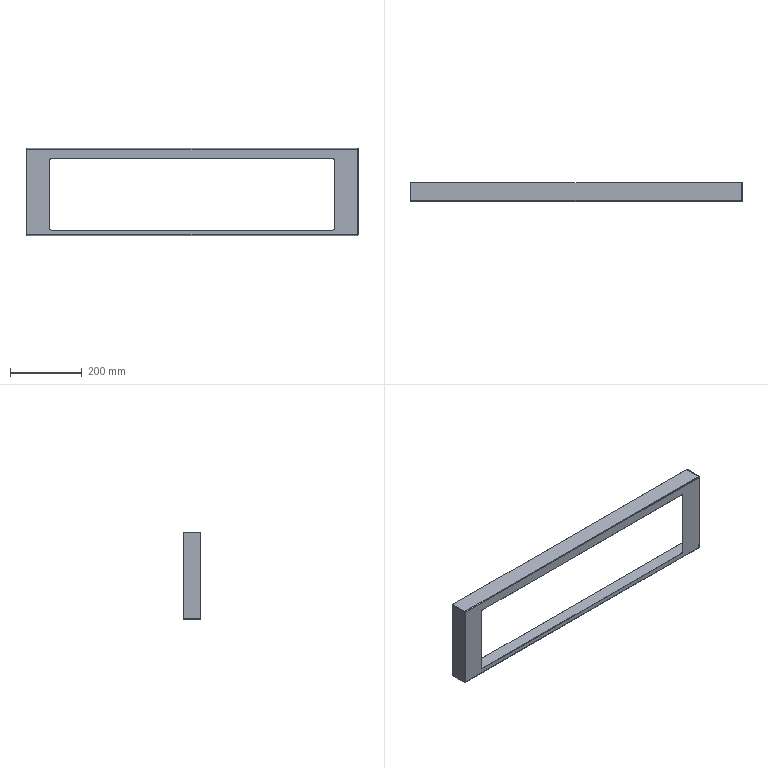Part | SolidWorks | features BaseBody 1 | 1 solid | 48 faces | box 927 x 50 x 243 mm | volume 213988 mm3 | plane 36 | cylinder 12 | commonest cylinder face diameters 2 x4 4.4 x4 10 x4
STEP:
#1=CARTESIAN_POINT('',(392.5,-23.8,13.8));
#2=VERTEX_POINT('',#1);
#3=CARTESIAN_POINT('',(397.5,-23.8,18.8));
#4=VERTEX_POINT('',#3);
#5=CARTESIAN_POINT('',(392.5,-23.8,18.8));
#6=DIRECTION('',(0.,-1.,0.));
#7=DIRECTION('',(0.,0.,1.));
#8=AXIS2_PLACEMENT_3D('',#5,#6,#7);
#9=CIRCLE('',#8,5.);
#10=EDGE_CURVE('',#2,#4,#9,.T.);
#11=ORIENTED_EDGE('',*,*,#10,.F.);
#12=CARTESIAN_POINT('',(392.5,-25.,13.8));
#13=VERTEX_POINT('',#12);
#14=CARTESIAN_POINT('',(392.5,-23.8,13.8));
#15=DIRECTION('',(0.,1.,0.));
#16=VECTOR('',#15,1000.);
#17=LINE('',#14,#16);
#18=EDGE_CURVE('',#13,#2,#17,.T.);
#19=ORIENTED_EDGE('',*,*,#18,.F.);
#20=CARTESIAN_POINT('',(397.5,-25.,18.8));
#21=VERTEX_POINT('',#20);
#22=CARTESIAN_POINT('',(392.5,-25.,18.8));
#23=DIRECTION('',(0.,1.,0.));
#24=DIRECTION('',(0.,0.,1.));
#25=AXIS2_PLACEMENT_3D('',#22,#23,#24);
#26=CIRCLE('',#25,5.);
#27=EDGE_CURVE('',#21,#13,#26,.T.);
#28=ORIENTED_EDGE('',*,*,#27,.F.);
#29=CARTESIAN_POINT('',(397.5,-25.,18.8));
#30=DIRECTION('',(0.,-1.,0.));
#31=VECTOR('',#30,1000.);
#32=LINE('',#29,#31);
#33=EDGE_CURVE('',#4,#21,#32,.T.);
#34=ORIENTED_EDGE('',*,*,#33,.F.);
#35=EDGE_LOOP('',(#11,#19,#28,#34));
#36=FACE_OUTER_BOUND('',#35,.T.);
#37=CARTESIAN_POINT('',(392.5,-15.,18.8));
#38=DIRECTION('',(0.,1.,0.));
#39=DIRECTION('',(0.,0.,1.));
#40=AXIS2_PLACEMENT_3D('',#37,#38,#39);
#41=CYLINDRICAL_SURFACE('',#40,5.);
#42=ADVANCED_FACE('',(#36),#41,.F.);
#43=CARTESIAN_POINT('',(-397.5,-23.8,18.8));
#44=VERTEX_POINT('',#43);
#45=CARTESIAN_POINT('',(-392.5,-23.8,13.8));
#46=VERTEX_POINT('',#45);
#47=CARTESIAN_POINT('',(-392.5,-23.8,18.8));
#48=DIRECTION('',(0.,-1.,0.));
#49=DIRECTION('',(0.,0.,1.));
#50=AXIS2_PLACEMENT_3D('',#47,#48,#49);
#51=CIRCLE('',#50,5.);
#52=EDGE_CURVE('',#44,#46,#51,.T.);
#53=ORIENTED_EDGE('',*,*,#52,.F.);
#54=CARTESIAN_POINT('',(-397.5,-25.,18.8));
#55=VERTEX_POINT('',#54);
#56=CARTESIAN_POINT('',(-397.5,-23.8,18.8));
#57=DIRECTION('',(0.,1.,0.));
#58=VECTOR('',#57,1000.);
#59=LINE('',#56,#58);
#60=EDGE_CURVE('',#55,#44,#59,.T.);
#61=ORIENTED_EDGE('',*,*,#60,.F.);
#62=CARTESIAN_POINT('',(-392.5,-25.,13.8));
#63=VERTEX_POINT('',#62);
#64=CARTESIAN_POINT('',(-392.5,-25.,18.8));
#65=DIRECTION('',(0.,1.,0.));
#66=DIRECTION('',(0.,0.,1.));
#67=AXIS2_PLACEMENT_3D('',#64,#65,#66);
#68=CIRCLE('',#67,5.);
#69=EDGE_CURVE('',#63,#55,#68,.T.);
#70=ORIENTED_EDGE('',*,*,#69,.F.);
#71=CARTESIAN_POINT('',(-392.5,-25.,13.8));
#72=DIRECTION('',(0.,-1.,0.));
#73=VECTOR('',#72,1000.);
#74=LINE('',#71,#73);
#75=EDGE_CURVE('',#46,#63,#74,.T.);
#76=ORIENTED_EDGE('',*,*,#75,.F.);
#77=EDGE_LOOP('',(#53,#61,#70,#76));
#78=FACE_OUTER_BOUND('',#77,.T.);
#79=CARTESIAN_POINT('',(-392.5,-15.,18.8));
#80=DIRECTION('',(0.,1.,0.));
#81=DIRECTION('',(0.,0.,1.));
#82=AXIS2_PLACEMENT_3D('',#79,#80,#81);
#83=CYLINDRICAL_SURFACE('',#82,5.);
#84=ADVANCED_FACE('',(#78),#83,.F.);
#85=CARTESIAN_POINT('',(-392.5,-23.8,213.8));
#86=VERTEX_POINT('',#85);
#87=CARTESIAN_POINT('',(-397.5,-23.8,208.8));
#88=VERTEX_POINT('',#87);
#89=CARTESIAN_POINT('',(-392.5,-23.8,208.8));
#90=DIRECTION('',(0.,-1.,0.));
#91=DIRECTION('',(0.,0.,1.));
#92=AXIS2_PLACEMENT_3D('',#89,#90,#91);
#93=CIRCLE('',#92,5.);
#94=EDGE_CURVE('',#86,#88,#93,.T.);
#95=ORIENTED_EDGE('',*,*,#94,.F.);
#96=CARTESIAN_POINT('',(-392.5,-25.,213.8));
#97=VERTEX_POINT('',#96);
#98=CARTESIAN_POINT('',(-392.5,-23.8,213.8));
#99=DIRECTION('',(0.,1.,0.));
#100=VECTOR('',#99,1000.);
#101=LINE('',#98,#100);
#102=EDGE_CURVE('',#97,#86,#101,.T.);
#103=ORIENTED_EDGE('',*,*,#102,.F.);
#104=CARTESIAN_POINT('',(-397.5,-25.,208.8));
#105=VERTEX_POINT('',#104);
#106=CARTESIAN_POINT('',(-392.5,-25.,208.8));
#107=DIRECTION('',(0.,1.,0.));
#108=DIRECTION('',(0.,0.,1.));
#109=AXIS2_PLACEMENT_3D('',#106,#107,#108);
#110=CIRCLE('',#109,5.);
#111=EDGE_CURVE('',#105,#97,#110,.T.);
#112=ORIENTED_EDGE('',*,*,#111,.F.);
#113=CARTESIAN_POINT('',(-397.5,-25.,208.8));
#114=DIRECTION('',(0.,-1.,0.));
#115=VECTOR('',#114,1000.);
#116=LINE('',#113,#115);
#117=EDGE_CURVE('',#88,#105,#116,.T.);
#118=ORIENTED_EDGE('',*,*,#117,.F.);
#119=EDGE_LOOP('',(#95,#103,#112,#118));
#120=FACE_OUTER_BOUND('',#119,.T.);
#121=CARTESIAN_POINT('',(-392.5,-15.,208.8));
#122=DIRECTION('',(0.,1.,0.));
#123=DIRECTION('',(0.,0.,1.));
#124=AXIS2_PLACEMENT_3D('',#121,#122,#123);
#125=CYLINDRICAL_SURFACE('',#124,5.);
#126=ADVANCED_FACE('',(#120),#125,.F.);
#127=CARTESIAN_POINT('',(397.5,-23.8,208.8));
#128=VERTEX_POINT('',#127);
#129=CARTESIAN_POINT('',(392.5,-23.8,213.8));
#130=VERTEX_POINT('',#129);
#131=CARTESIAN_POINT('',(392.5,-23.8,208.8));
#132=DIRECTION('',(0.,-1.,0.));
#133=DIRECTION('',(0.,0.,1.));
#134=AXIS2_PLACEMENT_3D('',#131,#132,#133);
#135=CIRCLE('',#134,5.);
#136=EDGE_CURVE('',#128,#130,#135,.T.);
#137=ORIENTED_EDGE('',*,*,#136,.F.);
#138=CARTESIAN_POINT('',(397.5,-25.,208.8));
#139=VERTEX_POINT('',#138);
#140=CARTESIAN_POINT('',(397.5,-23.8,208.8));
#141=DIRECTION('',(0.,1.,0.));
#142=VECTOR('',#141,1000.);
#143=LINE('',#140,#142);
#144=EDGE_CURVE('',#139,#128,#143,.T.);
#145=ORIENTED_EDGE('',*,*,#144,.F.);
#146=CARTESIAN_POINT('',(392.5,-25.,213.8));
#147=VERTEX_POINT('',#146);
#148=CARTESIAN_POINT('',(392.5,-25.,208.8));
#149=DIRECTION('',(0.,1.,0.));
#150=DIRECTION('',(0.,0.,1.));
#151=AXIS2_PLACEMENT_3D('',#148,#149,#150);
#152=CIRCLE('',#151,5.);
#153=EDGE_CURVE('',#147,#139,#152,.T.);
#154=ORIENTED_EDGE('',*,*,#153,.F.);
#155=CARTESIAN_POINT('',(392.5,-25.,213.8));
#156=DIRECTION('',(0.,-1.,0.));
#157=VECTOR('',#156,1000.);
#158=LINE('',#155,#157);
#159=EDGE_CURVE('',#130,#147,#158,.T.);
#160=ORIENTED_EDGE('',*,*,#159,.F.);
#161=EDGE_LOOP('',(#137,#145,#154,#160));
#162=FACE_OUTER_BOUND('',#161,.T.);
#163=CARTESIAN_POINT('',(392.5,-15.,208.8));
#164=DIRECTION('',(0.,1.,0.));
#165=DIRECTION('',(0.,0.,1.));
#166=AXIS2_PLACEMENT_3D('',#163,#164,#165);
#167=CYLINDRICAL_SURFACE('',#166,5.);
#168=ADVANCED_FACE('',(#162),#167,.F.);
#169=CARTESIAN_POINT('',(0.,-23.8,13.8));
#170=DIRECTION('',(-1.,0.,0.));
#171=VECTOR('',#170,1000.);
#172=LINE('',#169,#171);
#173=EDGE_CURVE('',#2,#46,#172,.T.);
#174=ORIENTED_EDGE('',*,*,#173,.T.);
#175=ORIENTED_EDGE('',*,*,#75,.T.);
#176=CARTESIAN_POINT('',(397.5,-25.,13.8));
#177=DIRECTION('',(1.,0.,0.));
#178=VECTOR('',#177,1000.);
#179=LINE('',#176,#178);
#180=EDGE_CURVE('',#63,#13,#179,.T.);
#181=ORIENTED_EDGE('',*,*,#180,.T.);
#182=ORIENTED_EDGE('',*,*,#18,.T.);
#183=EDGE_LOOP('',(#174,#175,#181,#182));
#184=FACE_OUTER_BOUND('',#183,.T.);
#185=CARTESIAN_POINT('',(397.5,-15.,13.8));
#186=DIRECTION('',(0.,0.,-1.));
#187=DIRECTION('',(-1.,0.,0.));
#188=AXIS2_PLACEMENT_3D('',#185,#186,#187);
#189=PLANE('',#188);
#190=ADVANCED_FACE('',(#184),#189,.F.);
#191=CARTESIAN_POINT('',(397.5,-25.,213.8));
#192=DIRECTION('',(0.,0.,1.));
#193=VECTOR('',#192,1000.);
#194=LINE('',#191,#193);
#195=EDGE_CURVE('',#21,#139,#194,.T.);
#196=ORIENTED_EDGE('',*,*,#195,.T.);
#197=ORIENTED_EDGE('',*,*,#144,.T.);
#198=CARTESIAN_POINT('',(397.5,-23.8,0.));
#199=DIRECTION('',(0.,0.,-1.));
#200=VECTOR('',#199,1000.);
#201=LINE('',#198,#200);
#202=EDGE_CURVE('',#128,#4,#201,.T.);
#203=ORIENTED_EDGE('',*,*,#202,.T.);
#204=ORIENTED_EDGE('',*,*,#33,.T.);
#205=EDGE_LOOP('',(#196,#197,#203,#204));
#206=FACE_OUTER_BOUND('',#205,.T.);
#207=CARTESIAN_POINT('',(397.5,-15.,213.8));
#208=DIRECTION('',(1.,0.,0.));
#209=DIRECTION('',(0.,1.,0.));
#210=AXIS2_PLACEMENT_3D('',#207,#208,#209);
#211=PLANE('',#210);
#212=ADVANCED_FACE('',(#206),#211,.F.);
#213=CARTESIAN_POINT('',(0.,-23.8,213.8));
#214=DIRECTION('',(1.,0.,0.));
#215=VECTOR('',#214,1000.);
#216=LINE('',#213,#215);
#217=EDGE_CURVE('',#86,#130,#216,.T.);
#218=ORIENTED_EDGE('',*,*,#217,.T.);
#219=ORIENTED_EDGE('',*,*,#159,.T.);
#220=CARTESIAN_POINT('',(397.5,-25.,213.8));
#221=DIRECTION('',(-1.,0.,0.));
#222=VECTOR('',#221,1000.);
#223=LINE('',#220,#222);
#224=EDGE_CURVE('',#147,#97,#223,.T.);
#225=ORIENTED_EDGE('',*,*,#224,.T.);
#226=ORIENTED_EDGE('',*,*,#102,.T.);
#227=EDGE_LOOP('',(#218,#219,#225,#226));
#228=FACE_OUTER_BOUND('',#227,.T.);
#229=CARTESIAN_POINT('',(397.5,-15.,213.8));
#230=DIRECTION('',(0.,0.,1.));
#231=DIRECTION('',(0.,-1.,0.));
#232=AXIS2_PLACEMENT_3D('',#229,#230,#231);
#233=PLANE('',#232);
#234=ADVANCED_FACE('',(#228),#233,.F.);
#235=CARTESIAN_POINT('',(-397.5,-23.8,0.));
#236=DIRECTION('',(0.,0.,1.));
#237=VECTOR('',#236,1000.);
#238=LINE('',#235,#237);
#239=EDGE_CURVE('',#44,#88,#238,.T.);
#240=ORIENTED_EDGE('',*,*,#239,.T.);
#241=ORIENTED_EDGE('',*,*,#117,.T.);
#242=CARTESIAN_POINT('',(-397.5,-25.,213.8));
#243=DIRECTION('',(0.,0.,-1.));
#244=VECTOR('',#243,1000.);
#245=LINE('',#242,#244);
#246=EDGE_CURVE('',#105,#55,#245,.T.);
#247=ORIENTED_EDGE('',*,*,#246,.T.);
#248=ORIENTED_EDGE('',*,*,#60,.T.);
#249=EDGE_LOOP('',(#240,#241,#247,#248));
#250=FACE_OUTER_BOUND('',#249,.T.);
#251=CARTESIAN_POINT('',(-397.5,-15.,213.8));
#252=DIRECTION('',(-1.,0.,0.));
#253=DIRECTION('',(0.,1.,0.));
#254=AXIS2_PLACEMENT_3D('',#251,#252,#253);
#255=PLANE('',#254);
#256=ADVANCED_FACE('',(#250),#255,.F.);
#257=CARTESIAN_POINT('',(461.3,25.,240.6));
#258=VERTEX_POINT('',#257);
#259=CARTESIAN_POINT('',(-461.3,25.,240.6));
#260=VERTEX_POINT('',#259);
#261=CARTESIAN_POINT('',(-461.3,25.,240.6));
#262=DIRECTION('',(-1.,0.,0.));
#263=VECTOR('',#262,1000.);
#264=LINE('',#261,#263);
#265=EDGE_CURVE('',#258,#260,#264,.T.);
#266=ORIENTED_EDGE('',*,*,#265,.T.);
#267=CARTESIAN_POINT('',(-461.3,25.,241.8));
#268=VERTEX_POINT('',#267);
#269=CARTESIAN_POINT('',(-461.3,25.,241.8));
#270=DIRECTION('',(0.,0.,-1.));
#271=VECTOR('',#270,1000.);
#272=LINE('',#269,#271);
#273=EDGE_CURVE('',#268,#260,#272,.T.);
#274=ORIENTED_EDGE('',*,*,#273,.F.);
#275=CARTESIAN_POINT('',(461.3,25.,241.8));
#276=VERTEX_POINT('',#275);
#277=CARTESIAN_POINT('',(0.,25.,241.8));
#278=DIRECTION('',(-1.,0.,0.));
#279=VECTOR('',#278,1000.);
#280=LINE('',#277,#279);
#281=EDGE_CURVE('',#276,#268,#280,.T.);
#282=ORIENTED_EDGE('',*,*,#281,.F.);
#283=CARTESIAN_POINT('',(461.3,25.,241.8));
#284=DIRECTION('',(0.,0.,-1.));
#285=VECTOR('',#284,1000.);
#286=LINE('',#283,#285);
#287=EDGE_CURVE('',#276,#258,#286,.T.);
#288=ORIENTED_EDGE('',*,*,#287,.T.);
#289=EDGE_LOOP('',(#266,#274,#282,#288));
#290=FACE_OUTER_BOUND('',#289,.T.);
#291=CARTESIAN_POINT('',(-461.3,25.,241.8));
#292=DIRECTION('',(0.,-1.,0.));
#293=DIRECTION('',(0.,0.,-1.));
#294=AXIS2_PLACEMENT_3D('',#291,#292,#293);
#295=PLANE('',#294);
#296=ADVANCED_FACE('',(#290),#295,.F.);
#297=CARTESIAN_POINT('',(461.3,-22.8,240.6));
#298=VERTEX_POINT('',#297);
#299=CARTESIAN_POINT('',(461.3,25.,240.6));
#300=DIRECTION('',(0.,1.,0.));
#301=VECTOR('',#300,1000.);
#302=LINE('',#299,#301);
#303=EDGE_CURVE('',#298,#258,#302,.T.);
#304=ORIENTED_EDGE('',*,*,#303,.F.);
#305=CARTESIAN_POINT('',(-461.3,-22.8,240.6));
#306=VERTEX_POINT('',#305);
#307=CARTESIAN_POINT('',(-461.3,-22.8,240.6));
#308=DIRECTION('',(1.,0.,0.));
#309=VECTOR('',#308,1000.);
#310=LINE('',#307,#309);
#311=EDGE_CURVE('',#306,#298,#310,.T.);
#312=ORIENTED_EDGE('',*,*,#311,.F.);
#313=CARTESIAN_POINT('',(-461.3,-23.8,240.6));
#314=DIRECTION('',(0.,-1.,0.));
#315=VECTOR('',#314,1000.);
#316=LINE('',#313,#315);
#317=EDGE_CURVE('',#260,#306,#316,.T.);
#318=ORIENTED_EDGE('',*,*,#317,.F.);
#319=ORIENTED_EDGE('',*,*,#265,.F.);
#320=EDGE_LOOP('',(#304,#312,#318,#319));
#321=FACE_OUTER_BOUND('',#320,.T.);
#322=CARTESIAN_POINT('',(0.,0.,240.6));
#323=DIRECTION('',(0.,0.,-1.));
#324=DIRECTION('',(0.,-1.,0.));
#325=AXIS2_PLACEMENT_3D('',#322,#323,#324);
#326=PLANE('',#325);
#327=ADVANCED_FACE('',(#321),#326,.T.);
#328=CARTESIAN_POINT('',(461.3,-22.8,241.8));
#329=VERTEX_POINT('',#328);
#330=CARTESIAN_POINT('',(-461.3,-22.8,241.8));
#331=VERTEX_POINT('',#330);
#332=CARTESIAN_POINT('',(-461.3,-22.8,241.8));
#333=DIRECTION('',(-1.,0.,0.));
#334=VECTOR('',#333,1000.);
#335=LINE('',#332,#334);
#336=EDGE_CURVE('',#329,#331,#335,.T.);
#337=ORIENTED_EDGE('',*,*,#336,.F.);
#338=CARTESIAN_POINT('',(461.3,0.,241.8));
#339=DIRECTION('',(0.,1.,0.));
#340=VECTOR('',#339,1000.);
#341=LINE('',#338,#340);
#342=EDGE_CURVE('',#329,#276,#341,.T.);
#343=ORIENTED_EDGE('',*,*,#342,.T.);
#344=ORIENTED_EDGE('',*,*,#281,.T.);
#345=CARTESIAN_POINT('',(-461.3,0.,241.8));
#346=DIRECTION('',(0.,-1.,0.));
#347=VECTOR('',#346,1000.);
#348=LINE('',#345,#347);
#349=EDGE_CURVE('',#268,#331,#348,.T.);
#350=ORIENTED_EDGE('',*,*,#349,.T.);
#351=EDGE_LOOP('',(#337,#343,#344,#350));
#352=FACE_OUTER_BOUND('',#351,.T.);
#353=CARTESIAN_POINT('',(0.,0.,241.8));
#354=DIRECTION('',(0.,0.,-1.));
#355=DIRECTION('',(0.,-1.,0.));
#356=AXIS2_PLACEMENT_3D('',#353,#354,#355);
#357=PLANE('',#356);
#358=ADVANCED_FACE('',(#352),#357,.F.);
#359=CARTESIAN_POINT('',(-461.3,-22.8,241.8));
#360=DIRECTION('',(0.,0.,1.));
#361=VECTOR('',#360,1000.);
#362=LINE('',#359,#361);
#363=EDGE_CURVE('',#306,#331,#362,.T.);
#364=ORIENTED_EDGE('',*,*,#363,.T.);
#365=ORIENTED_EDGE('',*,*,#349,.F.);
#366=ORIENTED_EDGE('',*,*,#273,.T.);
#367=ORIENTED_EDGE('',*,*,#317,.T.);
#368=EDGE_LOOP('',(#364,#365,#366,#367));
#369=FACE_OUTER_BOUND('',#368,.T.);
#370=CARTESIAN_POINT('',(-461.3,-23.8,241.8));
#371=DIRECTION('',(1.,0.,0.));
#372=DIRECTION('',(0.,1.,0.));
#373=AXIS2_PLACEMENT_3D('',#370,#371,#372);
#374=PLANE('',#373);
#375=ADVANCED_FACE('',(#369),#374,.F.);
#376=CARTESIAN_POINT('',(461.3,-22.8,240.6));
#377=DIRECTION('',(0.,0.,1.));
#378=VECTOR('',#377,1000.);
#379=LINE('',#376,#378);
#380=EDGE_CURVE('',#298,#329,#379,.T.);
#381=ORIENTED_EDGE('',*,*,#380,.F.);
#382=ORIENTED_EDGE('',*,*,#303,.T.);
#383=ORIENTED_EDGE('',*,*,#287,.F.);
#384=ORIENTED_EDGE('',*,*,#342,.F.);
#385=EDGE_LOOP('',(#381,#382,#383,#384));
#386=FACE_OUTER_BOUND('',#385,.T.);
#387=CARTESIAN_POINT('',(461.3,25.,241.8));
#388=DIRECTION('',(-1.,0.,0.));
#389=DIRECTION('',(0.,0.,1.));
#390=AXIS2_PLACEMENT_3D('',#387,#388,#389);
#391=PLANE('',#390);
#392=ADVANCED_FACE('',(#386),#391,.F.);
#393=CARTESIAN_POINT('',(461.3,-23.8,239.6));
#394=VERTEX_POINT('',#393);
#395=CARTESIAN_POINT('',(-461.3,-23.8,239.6));
#396=VERTEX_POINT('',#395);
#397=CARTESIAN_POINT('',(461.3,-23.8,239.6));
#398=DIRECTION('',(-1.,0.,0.));
#399=VECTOR('',#398,1000.);
#400=LINE('',#397,#399);
#401=EDGE_CURVE('',#394,#396,#400,.T.);
#402=ORIENTED_EDGE('',*,*,#401,.T.);
#403=CARTESIAN_POINT('',(-461.3,-22.8,239.6));
#404=DIRECTION('',(-1.,0.,0.));
#405=DIRECTION('',(0.,0.,-1.));
#406=AXIS2_PLACEMENT_3D('',#403,#404,#405);
#407=CIRCLE('',#406,1.);
#408=EDGE_CURVE('',#396,#306,#407,.T.);
#409=ORIENTED_EDGE('',*,*,#408,.T.);
#410=ORIENTED_EDGE('',*,*,#311,.T.);
#411=CARTESIAN_POINT('',(461.3,-22.8,239.6));
#412=DIRECTION('',(1.,0.,0.));
#413=DIRECTION('',(0.,0.,-1.));
#414=AXIS2_PLACEMENT_3D('',#411,#412,#413);
#415=CIRCLE('',#414,1.);
#416=EDGE_CURVE('',#298,#394,#415,.T.);
#417=ORIENTED_EDGE('',*,*,#416,.T.);
#418=EDGE_LOOP('',(#402,#409,#410,#417));
#419=FACE_OUTER_BOUND('',#418,.T.);
#420=CARTESIAN_POINT('',(461.3,-22.8,239.6));
#421=DIRECTION('',(1.,0.,0.));
#422=DIRECTION('',(0.,0.,1.));
#423=AXIS2_PLACEMENT_3D('',#420,#421,#422);
#424=CYLINDRICAL_SURFACE('',#423,1.);
#425=ADVANCED_FACE('',(#419),#424,.F.);
#426=CARTESIAN_POINT('',(461.3,-25.,239.6));
#427=VERTEX_POINT('',#426);
#428=CARTESIAN_POINT('',(-461.3,-25.,239.6));
#429=VERTEX_POINT('',#428);
#430=CARTESIAN_POINT('',(461.3,-25.,239.6));
#431=DIRECTION('',(-1.,0.,0.));
#432=VECTOR('',#431,1000.);
#433=LINE('',#430,#432);
#434=EDGE_CURVE('',#427,#429,#433,.T.);
#435=ORIENTED_EDGE('',*,*,#434,.F.);
#436=CARTESIAN_POINT('',(461.3,-22.8,239.6));
#437=DIRECTION('',(1.,0.,0.));
#438=DIRECTION('',(0.,0.,-1.));
#439=AXIS2_PLACEMENT_3D('',#436,#437,#438);
#440=CIRCLE('',#439,2.2);
#441=EDGE_CURVE('',#329,#427,#440,.T.);
#442=ORIENTED_EDGE('',*,*,#441,.F.);
#443=ORIENTED_EDGE('',*,*,#336,.T.);
#444=CARTESIAN_POINT('',(-461.3,-22.8,239.6));
#445=DIRECTION('',(-1.,0.,0.));
#446=DIRECTION('',(0.,0.,-1.));
#447=AXIS2_PLACEMENT_3D('',#444,#445,#446);
#448=CIRCLE('',#447,2.2);
#449=EDGE_CURVE('',#429,#331,#448,.T.);
#450=ORIENTED_EDGE('',*,*,#449,.F.);
#451=EDGE_LOOP('',(#435,#442,#443,#450));
#452=FACE_OUTER_BOUND('',#451,.T.);
#453=CARTESIAN_POINT('',(461.3,-22.8,239.6));
#454=DIRECTION('',(1.,0.,0.));
#455=DIRECTION('',(0.,0.,1.));
#456=AXIS2_PLACEMENT_3D('',#453,#454,#455);
#457=CYLINDRICAL_SURFACE('',#456,2.2);
#458=ADVANCED_FACE('',(#452),#457,.T.);
#459=ORIENTED_EDGE('',*,*,#416,.F.);
#460=ORIENTED_EDGE('',*,*,#380,.T.);
#461=ORIENTED_EDGE('',*,*,#441,.T.);
#462=CARTESIAN_POINT('',(461.3,-23.8,239.6));
#463=DIRECTION('',(0.,-1.,0.));
#464=VECTOR('',#463,1000.);
#465=LINE('',#462,#464);
#466=EDGE_CURVE('',#394,#427,#465,.T.);
#467=ORIENTED_EDGE('',*,*,#466,.F.);
#468=EDGE_LOOP('',(#459,#460,#461,#467));
#469=FACE_OUTER_BOUND('',#468,.T.);
#470=CARTESIAN_POINT('',(461.3,-22.8,239.6));
#471=DIRECTION('',(-1.,0.,0.));
#472=DIRECTION('',(0.,0.,1.));
#473=AXIS2_PLACEMENT_3D('',#470,#471,#472);
#474=PLANE('',#473);
#475=ADVANCED_FACE('',(#469),#474,.F.);
#476=ORIENTED_EDGE('',*,*,#363,.F.);
#477=ORIENTED_EDGE('',*,*,#408,.F.);
#478=CARTESIAN_POINT('',(-461.3,-23.8,239.6));
#479=DIRECTION('',(0.,-1.,0.));
#480=VECTOR('',#479,1000.);
#481=LINE('',#478,#480);
#482=EDGE_CURVE('',#396,#429,#481,.T.);
#483=ORIENTED_EDGE('',*,*,#482,.T.);
#484=ORIENTED_EDGE('',*,*,#449,.T.);
#485=EDGE_LOOP('',(#476,#477,#483,#484));
#486=FACE_OUTER_BOUND('',#485,.T.);
#487=CARTESIAN_POINT('',(-461.3,-22.8,239.6));
#488=DIRECTION('',(-1.,0.,0.));
#489=DIRECTION('',(0.,0.,1.));
#490=AXIS2_PLACEMENT_3D('',#487,#488,#489);
#491=PLANE('',#490);
#492=ADVANCED_FACE('',(#486),#491,.T.);
#493=CARTESIAN_POINT('',(461.3,-22.8,0.));
#494=VERTEX_POINT('',#493);
#495=CARTESIAN_POINT('',(-461.3,-22.8,0.));
#496=VERTEX_POINT('',#495);
#497=CARTESIAN_POINT('',(461.3,-22.8,0.));
#498=DIRECTION('',(-1.,0.,0.));
#499=VECTOR('',#498,1000.);
#500=LINE('',#497,#499);
#501=EDGE_CURVE('',#494,#496,#500,.T.);
#502=ORIENTED_EDGE('',*,*,#501,.T.);
#503=CARTESIAN_POINT('',(-461.3,-23.8,1.));
#504=VERTEX_POINT('',#503);
#505=CARTESIAN_POINT('',(-461.3,-22.8,1.));
#506=DIRECTION('',(-1.,0.,0.));
#507=DIRECTION('',(0.,0.,-1.));
#508=AXIS2_PLACEMENT_3D('',#505,#506,#507);
#509=CIRCLE('',#508,1.);
#510=EDGE_CURVE('',#496,#504,#509,.T.);
#511=ORIENTED_EDGE('',*,*,#510,.T.);
#512=CARTESIAN_POINT('',(461.3,-23.8,1.));
#513=VERTEX_POINT('',#512);
#514=CARTESIAN_POINT('',(-461.3,-23.8,1.));
#515=DIRECTION('',(1.,0.,0.));
#516=VECTOR('',#515,1000.);
#517=LINE('',#514,#516);
#518=EDGE_CURVE('',#504,#513,#517,.T.);
#519=ORIENTED_EDGE('',*,*,#518,.T.);
#520=CARTESIAN_POINT('',(461.3,-22.8,1.));
#521=DIRECTION('',(1.,0.,0.));
#522=DIRECTION('',(0.,0.,-1.));
#523=AXIS2_PLACEMENT_3D('',#520,#521,#522);
#524=CIRCLE('',#523,1.);
#525=EDGE_CURVE('',#513,#494,#524,.T.);
#526=ORIENTED_EDGE('',*,*,#525,.T.);
#527=EDGE_LOOP('',(#502,#511,#519,#526));
#528=FACE_OUTER_BOUND('',#527,.T.);
#529=CARTESIAN_POINT('',(461.3,-22.8,1.));
#530=DIRECTION('',(1.,0.,0.));
#531=DIRECTION('',(0.,-1.,0.));
#532=AXIS2_PLACEMENT_3D('',#529,#530,#531);
#533=CYLINDRICAL_SURFACE('',#532,1.);
#534=ADVANCED_FACE('',(#528),#533,.F.);
#535=CARTESIAN_POINT('',(461.3,-22.8,-1.2));
#536=VERTEX_POINT('',#535);
#537=CARTESIAN_POINT('',(-461.3,-22.8,-1.2));
#538=VERTEX_POINT('',#537);
#539=CARTESIAN_POINT('',(461.3,-22.8,-1.2));
#540=DIRECTION('',(-1.,0.,0.));
#541=VECTOR('',#540,1000.);
#542=LINE('',#539,#541);
#543=EDGE_CURVE('',#536,#538,#542,.T.);
#544=ORIENTED_EDGE('',*,*,#543,.F.);
#545=CARTESIAN_POINT('',(461.3,-24.76,0.));
#546=VERTEX_POINT('',#545);
#547=CARTESIAN_POINT('',(461.3,-22.8,1.));
#548=DIRECTION('',(1.,0.,0.));
#549=DIRECTION('',(0.,0.,-1.));
#550=AXIS2_PLACEMENT_3D('',#547,#548,#549);
#551=CIRCLE('',#550,2.2);
#552=EDGE_CURVE('',#546,#536,#551,.T.);
#553=ORIENTED_EDGE('',*,*,#552,.F.);
#554=CARTESIAN_POINT('',(461.3,-25.,1.));
#555=VERTEX_POINT('',#554);
#556=CARTESIAN_POINT('',(461.3,-22.8,1.));
#557=DIRECTION('',(1.,0.,0.));
#558=DIRECTION('',(0.,0.,-1.));
#559=AXIS2_PLACEMENT_3D('',#556,#557,#558);
#560=CIRCLE('',#559,2.2);
#561=EDGE_CURVE('',#555,#546,#560,.T.);
#562=ORIENTED_EDGE('',*,*,#561,.F.);
#563=CARTESIAN_POINT('',(-461.3,-25.,1.));
#564=VERTEX_POINT('',#563);
#565=CARTESIAN_POINT('',(-461.3,-25.,1.));
#566=DIRECTION('',(-1.,0.,0.));
#567=VECTOR('',#566,1000.);
#568=LINE('',#565,#567);
#569=EDGE_CURVE('',#555,#564,#568,.T.);
#570=ORIENTED_EDGE('',*,*,#569,.T.);
#571=CARTESIAN_POINT('',(-461.3,-24.76,0.));
#572=VERTEX_POINT('',#571);
#573=CARTESIAN_POINT('',(-461.3,-22.8,1.));
#574=DIRECTION('',(-1.,0.,0.));
#575=DIRECTION('',(0.,0.,-1.));
#576=AXIS2_PLACEMENT_3D('',#573,#574,#575);
#577=CIRCLE('',#576,2.2);
#578=EDGE_CURVE('',#572,#564,#577,.T.);
#579=ORIENTED_EDGE('',*,*,#578,.F.);
#580=CARTESIAN_POINT('',(-461.3,-22.8,1.));
#581=DIRECTION('',(-1.,0.,0.));
#582=DIRECTION('',(0.,0.,-1.));
#583=AXIS2_PLACEMENT_3D('',#580,#581,#582);
#584=CIRCLE('',#583,2.2);
#585=EDGE_CURVE('',#538,#572,#584,.T.);
#586=ORIENTED_EDGE('',*,*,#585,.F.);
#587=EDGE_LOOP('',(#544,#553,#562,#570,#579,#586));
#588=FACE_OUTER_BOUND('',#587,.T.);
#589=CARTESIAN_POINT('',(461.3,-22.8,1.));
#590=DIRECTION('',(1.,0.,0.));
#591=DIRECTION('',(0.,-1.,0.));
#592=AXIS2_PLACEMENT_3D('',#589,#590,#591);
#593=CYLINDRICAL_SURFACE('',#592,2.2);
#594=ADVANCED_FACE('',(#588),#593,.T.);
#595=ORIENTED_EDGE('',*,*,#561,.T.);
#596=CARTESIAN_POINT('',(461.3,-25.,0.));
#597=DIRECTION('',(0.,1.,0.));
#598=VECTOR('',#597,1000.);
#599=LINE('',#596,#598);
#600=EDGE_CURVE('',#546,#494,#599,.T.);
#601=ORIENTED_EDGE('',*,*,#600,.T.);
#602=ORIENTED_EDGE('',*,*,#525,.F.);
#603=CARTESIAN_POINT('',(461.3,-23.8,1.));
#604=DIRECTION('',(0.,-1.,0.));
#605=VECTOR('',#604,1000.);
#606=LINE('',#603,#605);
#607=EDGE_CURVE('',#513,#555,#606,.T.);
#608=ORIENTED_EDGE('',*,*,#607,.T.);
#609=EDGE_LOOP('',(#595,#601,#602,#608));
#610=FACE_OUTER_BOUND('',#609,.T.);
#611=CARTESIAN_POINT('',(461.3,-22.8,1.));
#612=DIRECTION('',(-1.,0.,0.));
#613=DIRECTION('',(0.,0.,1.));
#614=AXIS2_PLACEMENT_3D('',#611,#612,#613);
#615=PLANE('',#614);
#616=ADVANCED_FACE('',(#610),#615,.F.);
#617=CARTESIAN_POINT('',(-461.3,-25.,0.));
#618=DIRECTION('',(0.,1.,0.));
#619=VECTOR('',#618,1000.);
#620=LINE('',#617,#619);
#621=EDGE_CURVE('',#572,#496,#620,.T.);
#622=ORIENTED_EDGE('',*,*,#621,.F.);
#623=ORIENTED_EDGE('',*,*,#578,.T.);
#624=CARTESIAN_POINT('',(-461.3,-25.,1.));
#625=DIRECTION('',(0.,-1.,0.));
#626=VECTOR('',#625,1000.);
#627=LINE('',#624,#626);
#628=EDGE_CURVE('',#504,#564,#627,.T.);
#629=ORIENTED_EDGE('',*,*,#628,.F.);
#630=ORIENTED_EDGE('',*,*,#510,.F.);
#631=EDGE_LOOP('',(#622,#623,#629,#630));
#632=FACE_OUTER_BOUND('',#631,.T.);
#633=CARTESIAN_POINT('',(-461.3,-22.8,1.));
#634=DIRECTION('',(-1.,0.,0.));
#635=DIRECTION('',(0.,0.,1.));
#636=AXIS2_PLACEMENT_3D('',#633,#634,#635);
#637=PLANE('',#636);
#638=ADVANCED_FACE('',(#632),#637,.T.);
#639=CARTESIAN_POINT('',(462.3,25.,241.8));
#640=VERTEX_POINT('',#639);
#641=CARTESIAN_POINT('',(462.3,-25.,241.8));
#642=VERTEX_POINT('',#641);
#643=CARTESIAN_POINT('',(462.3,-25.,241.8));
#644=DIRECTION('',(0.,-1.,0.));
#645=VECTOR('',#644,1000.);
#646=LINE('',#643,#645);
#647=EDGE_CURVE('',#640,#642,#646,.T.);
#648=ORIENTED_EDGE('',*,*,#647,.T.);
#649=CARTESIAN_POINT('',(463.5,-25.,241.8));
#650=VERTEX_POINT('',#649);
#651=CARTESIAN_POINT('',(463.5,-25.,241.8));
#652=DIRECTION('',(-1.,0.,0.));
#653=VECTOR('',#652,1000.);
#654=LINE('',#651,#653);
#655=EDGE_CURVE('',#650,#642,#654,.T.);
#656=ORIENTED_EDGE('',*,*,#655,.F.);
#657=CARTESIAN_POINT('',(463.5,25.,241.8));
#658=VERTEX_POINT('',#657);
#659=CARTESIAN_POINT('',(463.5,0.,241.8));
#660=DIRECTION('',(0.,-1.,0.));
#661=VECTOR('',#660,1000.);
#662=LINE('',#659,#661);
#663=EDGE_CURVE('',#658,#650,#662,.T.);
#664=ORIENTED_EDGE('',*,*,#663,.F.);
#665=CARTESIAN_POINT('',(463.5,25.,241.8));
#666=DIRECTION('',(-1.,0.,0.));
#667=VECTOR('',#666,1000.);
#668=LINE('',#665,#667);
#669=EDGE_CURVE('',#658,#640,#668,.T.);
#670=ORIENTED_EDGE('',*,*,#669,.T.);
#671=EDGE_LOOP('',(#648,#656,#664,#670));
#672=FACE_OUTER_BOUND('',#671,.T.);
#673=CARTESIAN_POINT('',(463.5,-25.,241.8));
#674=DIRECTION('',(0.,0.,-1.));
#675=DIRECTION('',(-1.,0.,0.));
#676=AXIS2_PLACEMENT_3D('',#673,#674,#675);
#677=PLANE('',#676);
#678=ADVANCED_FACE('',(#672),#677,.F.);
#679=CARTESIAN_POINT('',(462.3,25.,1.));
#680=VERTEX_POINT('',#679);
#681=CARTESIAN_POINT('',(462.3,25.,241.8));
#682=DIRECTION('',(0.,0.,1.));
#683=VECTOR('',#682,1000.);
#684=LINE('',#681,#683);
#685=EDGE_CURVE('',#680,#640,#684,.T.);
#686=ORIENTED_EDGE('',*,*,#685,.F.);
#687=CARTESIAN_POINT('',(462.3,-25.,1.));
#688=VERTEX_POINT('',#687);
#689=CARTESIAN_POINT('',(462.3,-25.,1.));
#690=DIRECTION('',(0.,1.,0.));
#691=VECTOR('',#690,1000.);
#692=LINE('',#689,#691);
#693=EDGE_CURVE('',#688,#680,#692,.T.);
#694=ORIENTED_EDGE('',*,*,#693,.F.);
#695=CARTESIAN_POINT('',(462.3,-25.,0.));
#696=DIRECTION('',(0.,0.,-1.));
#697=VECTOR('',#696,1000.);
#698=LINE('',#695,#697);
#699=EDGE_CURVE('',#642,#688,#698,.T.);
#700=ORIENTED_EDGE('',*,*,#699,.F.);
#701=ORIENTED_EDGE('',*,*,#647,.F.);
#702=EDGE_LOOP('',(#686,#694,#700,#701));
#703=FACE_OUTER_BOUND('',#702,.T.);
#704=CARTESIAN_POINT('',(462.3,0.,0.));
#705=DIRECTION('',(-1.,0.,0.));
#706=DIRECTION('',(0.,1.,0.));
#707=AXIS2_PLACEMENT_3D('',#704,#705,#706);
#708=PLANE('',#707);
#709=ADVANCED_FACE('',(#703),#708,.T.);
#710=CARTESIAN_POINT('',(463.5,25.,1.));
#711=VERTEX_POINT('',#710);
#712=CARTESIAN_POINT('',(463.5,-25.,1.));
#713=VERTEX_POINT('',#712);
#714=CARTESIAN_POINT('',(463.5,-25.,1.));
#715=DIRECTION('',(0.,-1.,0.));
#716=VECTOR('',#715,1000.);
#717=LINE('',#714,#716);
#718=EDGE_CURVE('',#711,#713,#717,.T.);
#719=ORIENTED_EDGE('',*,*,#718,.F.);
#720=CARTESIAN_POINT('',(463.5,25.,0.));
#721=DIRECTION('',(0.,0.,1.));
#722=VECTOR('',#721,1000.);
#723=LINE('',#720,#722);
#724=EDGE_CURVE('',#711,#658,#723,.T.);
#725=ORIENTED_EDGE('',*,*,#724,.T.);
#726=ORIENTED_EDGE('',*,*,#663,.T.);
#727=CARTESIAN_POINT('',(463.5,-25.,0.));
#728=DIRECTION('',(0.,0.,-1.));
#729=VECTOR('',#728,1000.);
#730=LINE('',#727,#729);
#731=EDGE_CURVE('',#650,#713,#730,.T.);
#732=ORIENTED_EDGE('',*,*,#731,.T.);
#733=EDGE_LOOP('',(#719,#725,#726,#732));
#734=FACE_OUTER_BOUND('',#733,.T.);
#735=CARTESIAN_POINT('',(463.5,0.,0.));
#736=DIRECTION('',(-1.,0.,0.));
#737=DIRECTION('',(0.,1.,0.));
#738=AXIS2_PLACEMENT_3D('',#735,#736,#737);
#739=PLANE('',#738);
#740=ADVANCED_FACE('',(#734),#739,.F.);
#741=CARTESIAN_POINT('',(462.3,25.,1.));
#742=DIRECTION('',(1.,0.,0.));
#743=VECTOR('',#742,1000.);
#744=LINE('',#741,#743);
#745=EDGE_CURVE('',#680,#711,#744,.T.);
#746=ORIENTED_EDGE('',*,*,#745,.F.);
#747=ORIENTED_EDGE('',*,*,#685,.T.);
#748=ORIENTED_EDGE('',*,*,#669,.F.);
#749=ORIENTED_EDGE('',*,*,#724,.F.);
#750=EDGE_LOOP('',(#746,#747,#748,#749));
#751=FACE_OUTER_BOUND('',#750,.T.);
#752=CARTESIAN_POINT('',(463.5,25.,241.8));
#753=DIRECTION('',(0.,-1.,0.));
#754=DIRECTION('',(0.,0.,-1.));
#755=AXIS2_PLACEMENT_3D('',#752,#753,#754);
#756=PLANE('',#755);
#757=ADVANCED_FACE('',(#751),#756,.F.);
#758=CARTESIAN_POINT('',(463.5,-25.,1.));
#759=DIRECTION('',(1.,0.,0.));
#760=VECTOR('',#759,1000.);
#761=LINE('',#758,#760);
#762=EDGE_CURVE('',#688,#713,#761,.T.);
#763=ORIENTED_EDGE('',*,*,#762,.T.);
#764=ORIENTED_EDGE('',*,*,#731,.F.);
#765=ORIENTED_EDGE('',*,*,#655,.T.);
#766=ORIENTED_EDGE('',*,*,#699,.T.);
#767=EDGE_LOOP('',(#763,#764,#765,#766));
#768=FACE_OUTER_BOUND('',#767,.T.);
#769=CARTESIAN_POINT('',(463.5,-25.,0.));
#770=DIRECTION('',(0.,1.,0.));
#771=DIRECTION('',(0.,0.,-1.));
#772=AXIS2_PLACEMENT_3D('',#769,#770,#771);
#773=PLANE('',#772);
#774=ADVANCED_FACE('',(#768),#773,.F.);
#775=CARTESIAN_POINT('',(461.3,25.,0.));
#776=VERTEX_POINT('',#775);
#777=CARTESIAN_POINT('',(461.3,25.,0.));
#778=DIRECTION('',(0.,-1.,0.));
#779=VECTOR('',#778,1000.);
#780=LINE('',#777,#779);
#781=EDGE_CURVE('',#776,#494,#780,.T.);
#782=ORIENTED_EDGE('',*,*,#781,.T.);
#783=ORIENTED_EDGE('',*,*,#600,.F.);
#784=CARTESIAN_POINT('',(461.3,-25.,0.));
#785=VERTEX_POINT('',#784);
#786=CARTESIAN_POINT('',(461.3,-25.,0.));
#787=DIRECTION('',(0.,1.,0.));
#788=VECTOR('',#787,1000.);
#789=LINE('',#786,#788);
#790=EDGE_CURVE('',#785,#546,#789,.T.);
#791=ORIENTED_EDGE('',*,*,#790,.F.);
#792=CARTESIAN_POINT('',(461.3,-25.,1.));
#793=DIRECTION('',(0.,-1.,0.));
#794=DIRECTION('',(0.,0.,1.));
#795=AXIS2_PLACEMENT_3D('',#792,#793,#794);
#796=CIRCLE('',#795,1.);
#797=EDGE_CURVE('',#785,#688,#796,.T.);
#798=ORIENTED_EDGE('',*,*,#797,.T.);
#799=ORIENTED_EDGE('',*,*,#693,.T.);
#800=CARTESIAN_POINT('',(461.3,25.,1.));
#801=DIRECTION('',(0.,1.,0.));
#802=DIRECTION('',(0.,0.,1.));
#803=AXIS2_PLACEMENT_3D('',#800,#801,#802);
#804=CIRCLE('',#803,1.);
#805=EDGE_CURVE('',#680,#776,#804,.T.);
#806=ORIENTED_EDGE('',*,*,#805,.T.);
#807=EDGE_LOOP('',(#782,#783,#791,#798,#799,#806));
#808=FACE_OUTER_BOUND('',#807,.T.);
#809=CARTESIAN_POINT('',(461.3,25.,1.));
#810=DIRECTION('',(0.,1.,0.));
#811=DIRECTION('',(1.,0.,0.));
#812=AXIS2_PLACEMENT_3D('',#809,#810,#811);
#813=CYLINDRICAL_SURFACE('',#812,1.);
#814=ADVANCED_FACE('',(#808),#813,.F.);
#815=CARTESIAN_POINT('',(461.3,25.,-1.2));
#816=VERTEX_POINT('',#815);
#817=CARTESIAN_POINT('',(461.3,25.,-1.2));
#818=DIRECTION('',(0.,-1.,0.));
#819=VECTOR('',#818,1000.);
#820=LINE('',#817,#819);
#821=EDGE_CURVE('',#816,#536,#820,.T.);
#822=ORIENTED_EDGE('',*,*,#821,.F.);
#823=CARTESIAN_POINT('',(461.3,25.,1.));
#824=DIRECTION('',(0.,1.,0.));
#825=DIRECTION('',(0.,0.,1.));
#826=AXIS2_PLACEMENT_3D('',#823,#824,#825);
#827=CIRCLE('',#826,2.2);
#828=EDGE_CURVE('',#711,#816,#827,.T.);
#829=ORIENTED_EDGE('',*,*,#828,.F.);
#830=ORIENTED_EDGE('',*,*,#718,.T.);
#831=CARTESIAN_POINT('',(461.3,-25.,-1.2));
#832=VERTEX_POINT('',#831);
#833=CARTESIAN_POINT('',(461.3,-25.,1.));
#834=DIRECTION('',(0.,-1.,0.));
#835=DIRECTION('',(0.,0.,1.));
#836=AXIS2_PLACEMENT_3D('',#833,#834,#835);
#837=CIRCLE('',#836,2.2);
#838=EDGE_CURVE('',#832,#713,#837,.T.);
#839=ORIENTED_EDGE('',*,*,#838,.F.);
#840=CARTESIAN_POINT('',(461.3,25.,-1.2));
#841=DIRECTION('',(0.,1.,0.));
#842=VECTOR('',#841,1000.);
#843=LINE('',#840,#842);
#844=EDGE_CURVE('',#832,#536,#843,.T.);
#845=ORIENTED_EDGE('',*,*,#844,.T.);
#846=EDGE_LOOP('',(#822,#829,#830,#839,#845));
#847=FACE_OUTER_BOUND('',#846,.T.);
#848=CARTESIAN_POINT('',(461.3,25.,1.));
#849=DIRECTION('',(0.,1.,0.));
#850=DIRECTION('',(1.,0.,0.));
#851=AXIS2_PLACEMENT_3D('',#848,#849,#850);
#852=CYLINDRICAL_SURFACE('',#851,2.2);
#853=ADVANCED_FACE('',(#847),#852,.T.);
#854=ORIENTED_EDGE('',*,*,#805,.F.);
#855=ORIENTED_EDGE('',*,*,#745,.T.);
#856=ORIENTED_EDGE('',*,*,#828,.T.);
#857=CARTESIAN_POINT('',(461.3,25.,0.));
#858=DIRECTION('',(0.,0.,-1.));
#859=VECTOR('',#858,1000.);
#860=LINE('',#857,#859);
#861=EDGE_CURVE('',#776,#816,#860,.T.);
#862=ORIENTED_EDGE('',*,*,#861,.F.);
#863=EDGE_LOOP('',(#854,#855,#856,#862));
#864=FACE_OUTER_BOUND('',#863,.T.);
#865=CARTESIAN_POINT('',(461.3,25.,1.));
#866=DIRECTION('',(0.,-1.,0.));
#867=DIRECTION('',(0.,0.,-1.));
#868=AXIS2_PLACEMENT_3D('',#865,#866,#867);
#869=PLANE('',#868);
#870=ADVANCED_FACE('',(#864),#869,.F.);
#871=ORIENTED_EDGE('',*,*,#762,.F.);
#872=ORIENTED_EDGE('',*,*,#797,.F.);
#873=CARTESIAN_POINT('',(461.3,-25.,0.));
#874=DIRECTION('',(0.,0.,-1.));
#875=VECTOR('',#874,1000.);
#876=LINE('',#873,#875);
#877=EDGE_CURVE('',#785,#832,#876,.T.);
#878=ORIENTED_EDGE('',*,*,#877,.T.);
#879=ORIENTED_EDGE('',*,*,#838,.T.);
#880=EDGE_LOOP('',(#871,#872,#878,#879));
#881=FACE_OUTER_BOUND('',#880,.T.);
#882=CARTESIAN_POINT('',(461.3,-25.,1.));
#883=DIRECTION('',(0.,-1.,0.));
#884=DIRECTION('',(0.,0.,-1.));
#885=AXIS2_PLACEMENT_3D('',#882,#883,#884);
#886=PLANE('',#885);
#887=ADVANCED_FACE('',(#881),#886,.T.);
#888=CARTESIAN_POINT('',(-462.3,-25.,241.8));
#889=VERTEX_POINT('',#888);
#890=CARTESIAN_POINT('',(-462.3,25.,241.8));
#891=VERTEX_POINT('',#890);
#892=CARTESIAN_POINT('',(-462.3,25.,241.8));
#893=DIRECTION('',(0.,1.,0.));
#894=VECTOR('',#893,1000.);
#895=LINE('',#892,#894);
#896=EDGE_CURVE('',#889,#891,#895,.T.);
#897=ORIENTED_EDGE('',*,*,#896,.T.);
#898=CARTESIAN_POINT('',(-463.5,25.,241.8));
#899=VERTEX_POINT('',#898);
#900=CARTESIAN_POINT('',(-463.5,25.,241.8));
#901=DIRECTION('',(1.,0.,0.));
#902=VECTOR('',#901,1000.);
#903=LINE('',#900,#902);
#904=EDGE_CURVE('',#899,#891,#903,.T.);
#905=ORIENTED_EDGE('',*,*,#904,.F.);
#906=CARTESIAN_POINT('',(-463.5,-25.,241.8));
#907=VERTEX_POINT('',#906);
#908=CARTESIAN_POINT('',(-463.5,0.,241.8));
#909=DIRECTION('',(0.,1.,0.));
#910=VECTOR('',#909,1000.);
#911=LINE('',#908,#910);
#912=EDGE_CURVE('',#907,#899,#911,.T.);
#913=ORIENTED_EDGE('',*,*,#912,.F.);
#914=CARTESIAN_POINT('',(-463.5,-25.,241.8));
#915=DIRECTION('',(1.,0.,0.));
#916=VECTOR('',#915,1000.);
#917=LINE('',#914,#916);
#918=EDGE_CURVE('',#907,#889,#917,.T.);
#919=ORIENTED_EDGE('',*,*,#918,.T.);
#920=EDGE_LOOP('',(#897,#905,#913,#919));
#921=FACE_OUTER_BOUND('',#920,.T.);
#922=CARTESIAN_POINT('',(-463.5,25.,241.8));
#923=DIRECTION('',(0.,0.,-1.));
#924=DIRECTION('',(0.,-1.,0.));
#925=AXIS2_PLACEMENT_3D('',#922,#923,#924);
#926=PLANE('',#925);
#927=ADVANCED_FACE('',(#921),#926,.F.);
#928=CARTESIAN_POINT('',(-462.3,-25.,1.));
#929=VERTEX_POINT('',#928);
#930=CARTESIAN_POINT('',(-462.3,-25.,241.8));
#931=DIRECTION('',(0.,0.,1.));
#932=VECTOR('',#931,1000.);
#933=LINE('',#930,#932);
#934=EDGE_CURVE('',#929,#889,#933,.T.);
#935=ORIENTED_EDGE('',*,*,#934,.F.);
#936=CARTESIAN_POINT('',(-462.3,25.,1.));
#937=VERTEX_POINT('',#936);
#938=CARTESIAN_POINT('',(-462.3,25.,1.));
#939=DIRECTION('',(0.,-1.,0.));
#940=VECTOR('',#939,1000.);
#941=LINE('',#938,#940);
#942=EDGE_CURVE('',#937,#929,#941,.T.);
#943=ORIENTED_EDGE('',*,*,#942,.F.);
#944=CARTESIAN_POINT('',(-462.3,25.,0.));
#945=DIRECTION('',(0.,0.,-1.));
#946=VECTOR('',#945,1000.);
#947=LINE('',#944,#946);
#948=EDGE_CURVE('',#891,#937,#947,.T.);
#949=ORIENTED_EDGE('',*,*,#948,.F.);
#950=ORIENTED_EDGE('',*,*,#896,.F.);
#951=EDGE_LOOP('',(#935,#943,#949,#950));
#952=FACE_OUTER_BOUND('',#951,.T.);
#953=CARTESIAN_POINT('',(-462.3,0.,0.));
#954=DIRECTION('',(1.,0.,0.));
#955=DIRECTION('',(0.,0.,1.));
#956=AXIS2_PLACEMENT_3D('',#953,#954,#955);
#957=PLANE('',#956);
#958=ADVANCED_FACE('',(#952),#957,.T.);
#959=CARTESIAN_POINT('',(-463.5,-25.,1.));
#960=VERTEX_POINT('',#959);
#961=CARTESIAN_POINT('',(-463.5,25.,1.));
#962=VERTEX_POINT('',#961);
#963=CARTESIAN_POINT('',(-463.5,25.,1.));
#964=DIRECTION('',(0.,1.,0.));
#965=VECTOR('',#964,1000.);
#966=LINE('',#963,#965);
#967=EDGE_CURVE('',#960,#962,#966,.T.);
#968=ORIENTED_EDGE('',*,*,#967,.F.);
#969=CARTESIAN_POINT('',(-463.5,-25.,0.));
#970=DIRECTION('',(0.,0.,1.));
#971=VECTOR('',#970,1000.);
#972=LINE('',#969,#971);
#973=EDGE_CURVE('',#960,#907,#972,.T.);
#974=ORIENTED_EDGE('',*,*,#973,.T.);
#975=ORIENTED_EDGE('',*,*,#912,.T.);
#976=CARTESIAN_POINT('',(-463.5,25.,0.));
#977=DIRECTION('',(0.,0.,-1.));
#978=VECTOR('',#977,1000.);
#979=LINE('',#976,#978);
#980=EDGE_CURVE('',#899,#962,#979,.T.);
#981=ORIENTED_EDGE('',*,*,#980,.T.);
#982=EDGE_LOOP('',(#968,#974,#975,#981));
#983=FACE_OUTER_BOUND('',#982,.T.);
#984=CARTESIAN_POINT('',(-463.5,0.,0.));
#985=DIRECTION('',(1.,0.,0.));
#986=DIRECTION('',(0.,0.,1.));
#987=AXIS2_PLACEMENT_3D('',#984,#985,#986);
#988=PLANE('',#987);
#989=ADVANCED_FACE('',(#983),#988,.F.);
#990=CARTESIAN_POINT('',(-462.3,-25.,1.));
#991=DIRECTION('',(-1.,0.,0.));
#992=VECTOR('',#991,1000.);
#993=LINE('',#990,#992);
#994=EDGE_CURVE('',#929,#960,#993,.T.);
#995=ORIENTED_EDGE('',*,*,#994,.F.);
#996=ORIENTED_EDGE('',*,*,#934,.T.);
#997=ORIENTED_EDGE('',*,*,#918,.F.);
#998=ORIENTED_EDGE('',*,*,#973,.F.);
#999=EDGE_LOOP('',(#995,#996,#997,#998));
#1000=FACE_OUTER_BOUND('',#999,.T.);
#1001=CARTESIAN_POINT('',(-463.5,-25.,241.8));
#1002=DIRECTION('',(0.,1.,0.));
#1003=DIRECTION('',(0.,0.,-1.));
#1004=AXIS2_PLACEMENT_3D('',#1001,#1002,#1003);
#1005=PLANE('',#1004);
#1006=ADVANCED_FACE('',(#1000),#1005,.F.);
#1007=CARTESIAN_POINT('',(-463.5,25.,1.));
#1008=DIRECTION('',(-1.,0.,0.));
#1009=VECTOR('',#1008,1000.);
#1010=LINE('',#1007,#1009);
#1011=EDGE_CURVE('',#937,#962,#1010,.T.);
#1012=ORIENTED_EDGE('',*,*,#1011,.T.);
#1013=ORIENTED_EDGE('',*,*,#980,.F.);
#1014=ORIENTED_EDGE('',*,*,#904,.T.);
#1015=ORIENTED_EDGE('',*,*,#948,.T.);
#1016=EDGE_LOOP('',(#1012,#1013,#1014,#1015));
#1017=FACE_OUTER_BOUND('',#1016,.T.);
#1018=CARTESIAN_POINT('',(-463.5,25.,0.));
#1019=DIRECTION('',(0.,-1.,0.));
#1020=DIRECTION('',(0.,0.,-1.));
#1021=AXIS2_PLACEMENT_3D('',#1018,#1019,#1020);
#1022=PLANE('',#1021);
#1023=ADVANCED_FACE('',(#1017),#1022,.F.);
#1024=CARTESIAN_POINT('',(-461.3,-25.,0.));
#1025=VERTEX_POINT('',#1024);
#1026=CARTESIAN_POINT('',(-461.3,-25.,0.));
#1027=DIRECTION('',(0.,1.,0.));
#1028=VECTOR('',#1027,1000.);
#1029=LINE('',#1026,#1028);
#1030=EDGE_CURVE('',#1025,#572,#1029,.T.);
#1031=ORIENTED_EDGE('',*,*,#1030,.T.);
#1032=ORIENTED_EDGE('',*,*,#621,.T.);
#1033=CARTESIAN_POINT('',(-461.3,25.,0.));
#1034=VERTEX_POINT('',#1033);
#1035=CARTESIAN_POINT('',(-461.3,-25.,0.));
#1036=DIRECTION('',(0.,1.,0.));
#1037=VECTOR('',#1036,1000.);
#1038=LINE('',#1035,#1037);
#1039=EDGE_CURVE('',#496,#1034,#1038,.T.);
#1040=ORIENTED_EDGE('',*,*,#1039,.T.);
#1041=CARTESIAN_POINT('',(-461.3,25.,1.));
#1042=DIRECTION('',(0.,1.,0.));
#1043=DIRECTION('',(0.,0.,-1.));
#1044=AXIS2_PLACEMENT_3D('',#1041,#1042,#1043);
#1045=CIRCLE('',#1044,1.);
#1046=EDGE_CURVE('',#1034,#937,#1045,.T.);
#1047=ORIENTED_EDGE('',*,*,#1046,.T.);
#1048=ORIENTED_EDGE('',*,*,#942,.T.);
#1049=CARTESIAN_POINT('',(-461.3,-25.,1.));
#1050=DIRECTION('',(0.,-1.,0.));
#1051=DIRECTION('',(0.,0.,-1.));
#1052=AXIS2_PLACEMENT_3D('',#1049,#1050,#1051);
#1053=CIRCLE('',#1052,1.);
#1054=EDGE_CURVE('',#929,#1025,#1053,.T.);
#1055=ORIENTED_EDGE('',*,*,#1054,.T.);
#1056=EDGE_LOOP('',(#1031,#1032,#1040,#1047,#1048,#1055));
#1057=FACE_OUTER_BOUND('',#1056,.T.);
#1058=CARTESIAN_POINT('',(-461.3,-25.,1.));
#1059=DIRECTION('',(0.,-1.,0.));
#1060=DIRECTION('',(-1.,0.,0.));
#1061=AXIS2_PLACEMENT_3D('',#1058,#1059,#1060);
#1062=CYLINDRICAL_SURFACE('',#1061,1.);
#1063=ADVANCED_FACE('',(#1057),#1062,.F.);
#1064=CARTESIAN_POINT('',(-461.3,-25.,-1.2));
#1065=VERTEX_POINT('',#1064);
#1066=CARTESIAN_POINT('',(-461.3,-25.,-1.2));
#1067=DIRECTION('',(0.,1.,0.));
#1068=VECTOR('',#1067,1000.);
#1069=LINE('',#1066,#1068);
#1070=EDGE_CURVE('',#1065,#538,#1069,.T.);
#1071=ORIENTED_EDGE('',*,*,#1070,.F.);
#1072=CARTESIAN_POINT('',(-461.3,-25.,1.));
#1073=DIRECTION('',(0.,-1.,0.));
#1074=DIRECTION('',(0.,0.,-1.));
#1075=AXIS2_PLACEMENT_3D('',#1072,#1073,#1074);
#1076=CIRCLE('',#1075,2.2);
#1077=EDGE_CURVE('',#960,#1065,#1076,.T.);
#1078=ORIENTED_EDGE('',*,*,#1077,.F.);
#1079=ORIENTED_EDGE('',*,*,#967,.T.);
#1080=CARTESIAN_POINT('',(-461.3,25.,-1.2));
#1081=VERTEX_POINT('',#1080);
#1082=CARTESIAN_POINT('',(-461.3,25.,1.));
#1083=DIRECTION('',(0.,1.,0.));
#1084=DIRECTION('',(0.,0.,-1.));
#1085=AXIS2_PLACEMENT_3D('',#1082,#1083,#1084);
#1086=CIRCLE('',#1085,2.2);
#1087=EDGE_CURVE('',#1081,#962,#1086,.T.);
#1088=ORIENTED_EDGE('',*,*,#1087,.F.);
#1089=CARTESIAN_POINT('',(-461.3,-25.,-1.2));
#1090=DIRECTION('',(0.,1.,0.));
#1091=VECTOR('',#1090,1000.);
#1092=LINE('',#1089,#1091);
#1093=EDGE_CURVE('',#538,#1081,#1092,.T.);
#1094=ORIENTED_EDGE('',*,*,#1093,.F.);
#1095=EDGE_LOOP('',(#1071,#1078,#1079,#1088,#1094));
#1096=FACE_OUTER_BOUND('',#1095,.T.);
#1097=CARTESIAN_POINT('',(-461.3,-25.,1.));
#1098=DIRECTION('',(0.,-1.,0.));
#1099=DIRECTION('',(-1.,0.,0.));
#1100=AXIS2_PLACEMENT_3D('',#1097,#1098,#1099);
#1101=CYLINDRICAL_SURFACE('',#1100,2.2);
#1102=ADVANCED_FACE('',(#1096),#1101,.T.);
#1103=ORIENTED_EDGE('',*,*,#1054,.F.);
#1104=ORIENTED_EDGE('',*,*,#994,.T.);
#1105=ORIENTED_EDGE('',*,*,#1077,.T.);
#1106=CARTESIAN_POINT('',(-461.3,-25.,0.));
#1107=DIRECTION('',(0.,0.,-1.));
#1108=VECTOR('',#1107,1000.);
#1109=LINE('',#1106,#1108);
#1110=EDGE_CURVE('',#1025,#1065,#1109,.T.);
#1111=ORIENTED_EDGE('',*,*,#1110,.F.);
#1112=EDGE_LOOP('',(#1103,#1104,#1105,#1111));
#1113=FACE_OUTER_BOUND('',#1112,.T.);
#1114=CARTESIAN_POINT('',(-461.3,-25.,1.));
#1115=DIRECTION('',(0.,1.,0.));
#1116=DIRECTION('',(1.,0.,0.));
#1117=AXIS2_PLACEMENT_3D('',#1114,#1115,#1116);
#1118=PLANE('',#1117);
#1119=ADVANCED_FACE('',(#1113),#1118,.F.);
#1120=ORIENTED_EDGE('',*,*,#1011,.F.);
#1121=ORIENTED_EDGE('',*,*,#1046,.F.);
#1122=CARTESIAN_POINT('',(-461.3,25.,0.));
#1123=DIRECTION('',(0.,0.,-1.));
#1124=VECTOR('',#1123,1000.);
#1125=LINE('',#1122,#1124);
#1126=EDGE_CURVE('',#1034,#1081,#1125,.T.);
#1127=ORIENTED_EDGE('',*,*,#1126,.T.);
#1128=ORIENTED_EDGE('',*,*,#1087,.T.);
#1129=EDGE_LOOP('',(#1120,#1121,#1127,#1128));
#1130=FACE_OUTER_BOUND('',#1129,.T.);
#1131=CARTESIAN_POINT('',(-461.3,25.,1.));
#1132=DIRECTION('',(0.,1.,0.));
#1133=DIRECTION('',(1.,0.,0.));
#1134=AXIS2_PLACEMENT_3D('',#1131,#1132,#1133);
#1135=PLANE('',#1134);
#1136=ADVANCED_FACE('',(#1130),#1135,.T.);
#1137=CARTESIAN_POINT('',(463.5,25.,0.));
#1138=DIRECTION('',(-1.,0.,0.));
#1139=VECTOR('',#1138,1000.);
#1140=LINE('',#1137,#1139);
#1141=EDGE_CURVE('',#776,#1034,#1140,.T.);
#1142=ORIENTED_EDGE('',*,*,#1141,.F.);
#1143=ORIENTED_EDGE('',*,*,#861,.T.);
#1144=CARTESIAN_POINT('',(463.5,25.,-1.2));
#1145=DIRECTION('',(-1.,0.,0.));
#1146=VECTOR('',#1145,1000.);
#1147=LINE('',#1144,#1146);
#1148=EDGE_CURVE('',#816,#1081,#1147,.T.);
#1149=ORIENTED_EDGE('',*,*,#1148,.T.);
#1150=ORIENTED_EDGE('',*,*,#1126,.F.);
#1151=EDGE_LOOP('',(#1142,#1143,#1149,#1150));
#1152=FACE_OUTER_BOUND('',#1151,.T.);
#1153=CARTESIAN_POINT('',(463.5,25.,-1.2));
#1154=DIRECTION('',(0.,1.,0.));
#1155=DIRECTION('',(1.,0.,0.));
#1156=AXIS2_PLACEMENT_3D('',#1153,#1154,#1155);
#1157=PLANE('',#1156);
#1158=ADVANCED_FACE('',(#1152),#1157,.T.);
#1159=ORIENTED_EDGE('',*,*,#501,.F.);
#1160=ORIENTED_EDGE('',*,*,#781,.F.);
#1161=ORIENTED_EDGE('',*,*,#1141,.T.);
#1162=ORIENTED_EDGE('',*,*,#1039,.F.);
#1163=EDGE_LOOP('',(#1159,#1160,#1161,#1162));
#1164=FACE_OUTER_BOUND('',#1163,.T.);
#1165=CARTESIAN_POINT('',(0.,0.,0.));
#1166=DIRECTION('',(0.,0.,-1.));
#1167=DIRECTION('',(0.,-1.,0.));
#1168=AXIS2_PLACEMENT_3D('',#1165,#1166,#1167);
#1169=PLANE('',#1168);
#1170=ADVANCED_FACE('',(#1164),#1169,.F.);
#1171=ORIENTED_EDGE('',*,*,#821,.T.);
#1172=ORIENTED_EDGE('',*,*,#543,.T.);
#1173=ORIENTED_EDGE('',*,*,#1093,.T.);
#1174=ORIENTED_EDGE('',*,*,#1148,.F.);
#1175=EDGE_LOOP('',(#1171,#1172,#1173,#1174));
#1176=FACE_OUTER_BOUND('',#1175,.T.);
#1177=CARTESIAN_POINT('',(0.,0.,-1.2));
#1178=DIRECTION('',(0.,0.,-1.));
#1179=DIRECTION('',(0.,-1.,0.));
#1180=AXIS2_PLACEMENT_3D('',#1177,#1178,#1179);
#1181=PLANE('',#1180);
#1182=ADVANCED_FACE('',(#1176),#1181,.T.);
#1183=ORIENTED_EDGE('',*,*,#1070,.T.);
#1184=ORIENTED_EDGE('',*,*,#585,.T.);
#1185=ORIENTED_EDGE('',*,*,#1030,.F.);
#1186=ORIENTED_EDGE('',*,*,#1110,.T.);
#1187=EDGE_LOOP('',(#1183,#1184,#1185,#1186));
#1188=FACE_OUTER_BOUND('',#1187,.T.);
#1189=CARTESIAN_POINT('',(-461.3,-22.8,0.));
#1190=DIRECTION('',(1.,0.,0.));
#1191=DIRECTION('',(0.,1.,0.));
#1192=AXIS2_PLACEMENT_3D('',#1189,#1190,#1191);
#1193=PLANE('',#1192);
#1194=ADVANCED_FACE('',(#1188),#1193,.T.);
#1195=ORIENTED_EDGE('',*,*,#790,.T.);
#1196=ORIENTED_EDGE('',*,*,#552,.T.);
#1197=ORIENTED_EDGE('',*,*,#844,.F.);
#1198=ORIENTED_EDGE('',*,*,#877,.F.);
#1199=EDGE_LOOP('',(#1195,#1196,#1197,#1198));
#1200=FACE_OUTER_BOUND('',#1199,.T.);
#1201=CARTESIAN_POINT('',(461.3,-25.,0.));
#1202=DIRECTION('',(-1.,0.,0.));
#1203=DIRECTION('',(0.,0.,1.));
#1204=AXIS2_PLACEMENT_3D('',#1201,#1202,#1203);
#1205=PLANE('',#1204);
#1206=ADVANCED_FACE('',(#1200),#1205,.T.);
#1207=ORIENTED_EDGE('',*,*,#239,.F.);
#1208=ORIENTED_EDGE('',*,*,#52,.T.);
#1209=ORIENTED_EDGE('',*,*,#173,.F.);
#1210=ORIENTED_EDGE('',*,*,#10,.T.);
#1211=ORIENTED_EDGE('',*,*,#202,.F.);
#1212=ORIENTED_EDGE('',*,*,#136,.T.);
#1213=ORIENTED_EDGE('',*,*,#217,.F.);
#1214=ORIENTED_EDGE('',*,*,#94,.T.);
#1215=EDGE_LOOP('',(#1207,#1208,#1209,#1210,#1211,#1212,#1213,#1214));
#1216=FACE_BOUND('',#1215,.T.);
#1217=CARTESIAN_POINT('',(-461.3,-23.8,0.));
#1218=DIRECTION('',(0.,0.,-1.));
#1219=VECTOR('',#1218,1000.);
#1220=LINE('',#1217,#1219);
#1221=EDGE_CURVE('',#396,#504,#1220,.T.);
#1222=ORIENTED_EDGE('',*,*,#1221,.F.);
#1223=ORIENTED_EDGE('',*,*,#401,.F.);
#1224=CARTESIAN_POINT('',(461.3,-23.8,241.8));
#1225=DIRECTION('',(0.,0.,1.));
#1226=VECTOR('',#1225,1000.);
#1227=LINE('',#1224,#1226);
#1228=EDGE_CURVE('',#513,#394,#1227,.T.);
#1229=ORIENTED_EDGE('',*,*,#1228,.F.);
#1230=ORIENTED_EDGE('',*,*,#518,.F.);
#1231=EDGE_LOOP('',(#1222,#1223,#1229,#1230));
#1232=FACE_OUTER_BOUND('',#1231,.T.);
#1233=CARTESIAN_POINT('',(0.,-23.8,0.));
#1234=DIRECTION('',(0.,1.,0.));
#1235=DIRECTION('',(0.,0.,-1.));
#1236=AXIS2_PLACEMENT_3D('',#1233,#1234,#1235);
#1237=PLANE('',#1236);
#1238=ADVANCED_FACE('',(#1216,#1232),#1237,.T.);
#1239=ORIENTED_EDGE('',*,*,#180,.F.);
#1240=ORIENTED_EDGE('',*,*,#69,.T.);
#1241=ORIENTED_EDGE('',*,*,#246,.F.);
#1242=ORIENTED_EDGE('',*,*,#111,.T.);
#1243=ORIENTED_EDGE('',*,*,#224,.F.);
#1244=ORIENTED_EDGE('',*,*,#153,.T.);
#1245=ORIENTED_EDGE('',*,*,#195,.F.);
#1246=ORIENTED_EDGE('',*,*,#27,.T.);
#1247=EDGE_LOOP('',(#1239,#1240,#1241,#1242,#1243,#1244,#1245,#1246));
#1248=FACE_BOUND('',#1247,.T.);
#1249=ORIENTED_EDGE('',*,*,#434,.T.);
#1250=CARTESIAN_POINT('',(-461.3,-25.,0.));
#1251=DIRECTION('',(0.,0.,-1.));
#1252=VECTOR('',#1251,1000.);
#1253=LINE('',#1250,#1252);
#1254=EDGE_CURVE('',#429,#564,#1253,.T.);
#1255=ORIENTED_EDGE('',*,*,#1254,.T.);
#1256=ORIENTED_EDGE('',*,*,#569,.F.);
#1257=CARTESIAN_POINT('',(461.3,-25.,0.));
#1258=DIRECTION('',(0.,0.,1.));
#1259=VECTOR('',#1258,1000.);
#1260=LINE('',#1257,#1259);
#1261=EDGE_CURVE('',#555,#427,#1260,.T.);
#1262=ORIENTED_EDGE('',*,*,#1261,.T.);
#1263=EDGE_LOOP('',(#1249,#1255,#1256,#1262));
#1264=FACE_OUTER_BOUND('',#1263,.T.);
#1265=CARTESIAN_POINT('',(0.,-25.,0.));
#1266=DIRECTION('',(0.,1.,0.));
#1267=DIRECTION('',(0.,0.,-1.));
#1268=AXIS2_PLACEMENT_3D('',#1265,#1266,#1267);
#1269=PLANE('',#1268);
#1270=ADVANCED_FACE('',(#1248,#1264),#1269,.F.);
#1271=ORIENTED_EDGE('',*,*,#466,.T.);
#1272=ORIENTED_EDGE('',*,*,#1261,.F.);
#1273=ORIENTED_EDGE('',*,*,#607,.F.);
#1274=ORIENTED_EDGE('',*,*,#1228,.T.);
#1275=EDGE_LOOP('',(#1271,#1272,#1273,#1274));
#1276=FACE_OUTER_BOUND('',#1275,.T.);
#1277=CARTESIAN_POINT('',(461.3,-25.,241.8));
#1278=DIRECTION('',(-1.,0.,0.));
#1279=DIRECTION('',(0.,1.,0.));
#1280=AXIS2_PLACEMENT_3D('',#1277,#1278,#1279);
#1281=PLANE('',#1280);
#1282=ADVANCED_FACE('',(#1276),#1281,.F.);
#1283=ORIENTED_EDGE('',*,*,#482,.F.);
#1284=ORIENTED_EDGE('',*,*,#1221,.T.);
#1285=ORIENTED_EDGE('',*,*,#628,.T.);
#1286=ORIENTED_EDGE('',*,*,#1254,.F.);
#1287=EDGE_LOOP('',(#1283,#1284,#1285,#1286));
#1288=FACE_OUTER_BOUND('',#1287,.T.);
#1289=CARTESIAN_POINT('',(-461.3,-25.,0.));
#1290=DIRECTION('',(1.,0.,0.));
#1291=DIRECTION('',(0.,1.,0.));
#1292=AXIS2_PLACEMENT_3D('',#1289,#1290,#1291);
#1293=PLANE('',#1292);
#1294=ADVANCED_FACE('',(#1288),#1293,.F.);
#1295=CLOSED_SHELL('',(#42,#84,#126,#168,#190,#212,#234,#256,#296,#327,#358,#375,#392,#425,#458,#475,#492,#534,#594,#616,#638,#678,#709,#740,#757,#774,#814,#853,#870,#887,#927,#958,#989,#1006,#1023,#1063,#1102,#1119,#1136,#1158,#1170,#1182,#1194,#1206,#1238,#1270,#1282,#1294));
#1296=MANIFOLD_SOLID_BREP('',#1295);
#1297=CARTESIAN_POINT('',(0.,0.,0.));
#1298=DIRECTION('',(0.,0.,1.));
#1299=DIRECTION('',(1.,0.,0.));
#1300=AXIS2_PLACEMENT_3D('',#1297,#1298,#1299);
#1301=(LENGTH_UNIT()NAMED_UNIT(*)SI_UNIT(.MILLI.,.METRE.));
#1302=UNCERTAINTY_MEASURE_WITH_UNIT(LENGTH_MEASURE(0.00001),#1301,'','');
#1303=(NAMED_UNIT(*)PLANE_ANGLE_UNIT()SI_UNIT($,.RADIAN.));
#1304=(NAMED_UNIT(*)SI_UNIT($,.STERADIAN.)SOLID_ANGLE_UNIT());
#1305=(GEOMETRIC_REPRESENTATION_CONTEXT(3)GLOBAL_UNCERTAINTY_ASSIGNED_CONTEXT((#1302))GLOBAL_UNIT_ASSIGNED_CONTEXT((#1301,#1303,#1304))REPRESENTATION_CONTEXT('',''));
#1306=ADVANCED_BREP_SHAPE_REPRESENTATION('',(#1296,#1300),#1305);